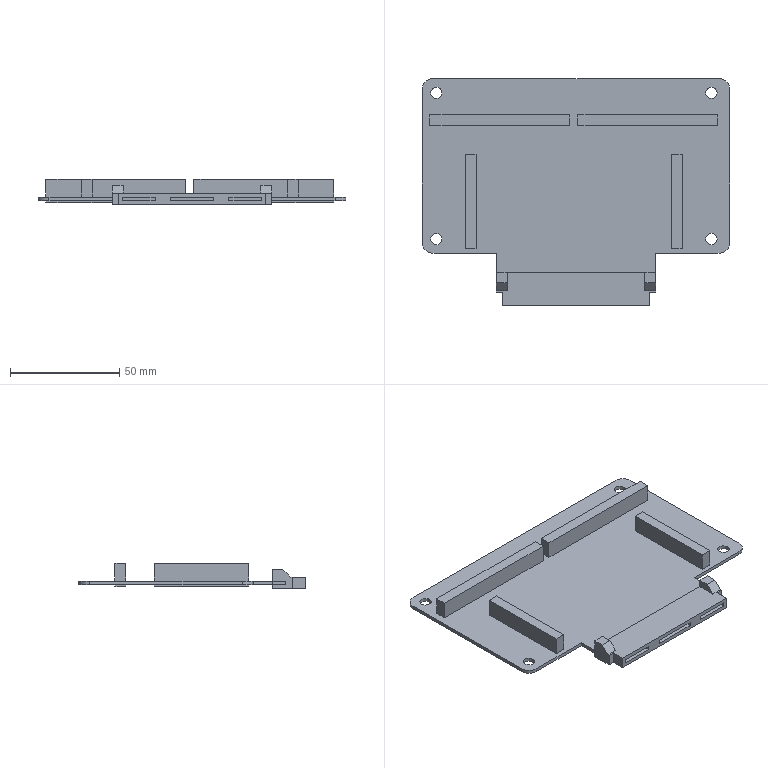Part | SolidWorks | features ICE 6, Attribute 3, Chamfer 1, Extrusion 1, Fillet 1 | 2 solids | 93 faces | box 141 x 103.9 x 11.65 mm | volume 34757 mm3 | plane 81 | cylinder 12 | commonest cylinder face diameters 5.2 x8 10 x4